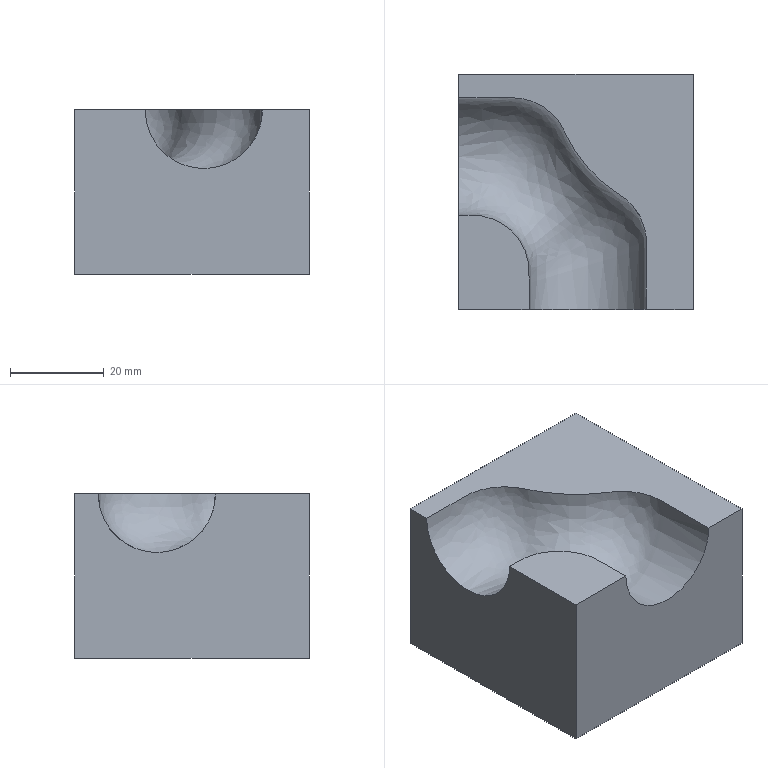CAM job | NX | 3-axis milling | part box 50 x 50 x 35 mm | stock box 50 x 50 x 35 mm
Tools:
number,name,description,diameter,corner_radius,flute_length,length,flutes
0,D12,Milling Tool-5 Parameters,12.0,0.0,50.0,75.0,2
0,D6,Milling Tool-5 Parameters,6.0,0.0,50.0,75.0,2
0,B8,Milling Tool-Ball Mill,8.0,4.0,50.0,75.0,2
Operations:
program,operation,operation_type,tool,method,geometry_group,spindle_rpm,surface_speed,feed_per_tooth,feed_cut,feed_plunge,cut_length_mm,path_length_mm,cut_time_min,machine_time_min
NC_PROGRAM,CAVITY_MILL,CavityMilling,D12,METHOD,WORKPIECE,3000.0,282.0,0.4167,2500.0,100.0,5714.148,6033.734,2.286,2.318
NC_PROGRAM,CAVITY_MILL_COPY,CavityMilling,D6,METHOD,WORKPIECE,3000.0,282.0,0.4167,2500.0,100.0,9114.168,11639.147,3.646,3.898
NC_PROGRAM,CAVITY_MILL_COPY_COPY,CavityMilling,B8,METHOD,WORKPIECE,3000.0,282.0,0.4167,2500.0,100.0,3700.878,4485.254,1.48,1.559
NC_PROGRAM,CONTOUR_AREA,SurfaceContour,B8,METHOD,WORKPIECE,3000.0,282.0,0.4167,2500.0,100.0,7654.23,7676.786,3.062,3.064
NC_PROGRAM,CONTOUR_AREA_1,SurfaceContour,B8,METHOD,WORKPIECE,3000.0,282.0,0.4167,2500.0,100.0,8840.782,9072.374,3.536,3.559
NC_PROGRAM,CONTOUR_AREA_1_COPY,SurfaceContour,B8,METHOD,WORKPIECE,3000.0,282.0,0.4167,2500.0,100.0,10716.679,10916.268,4.287,4.307